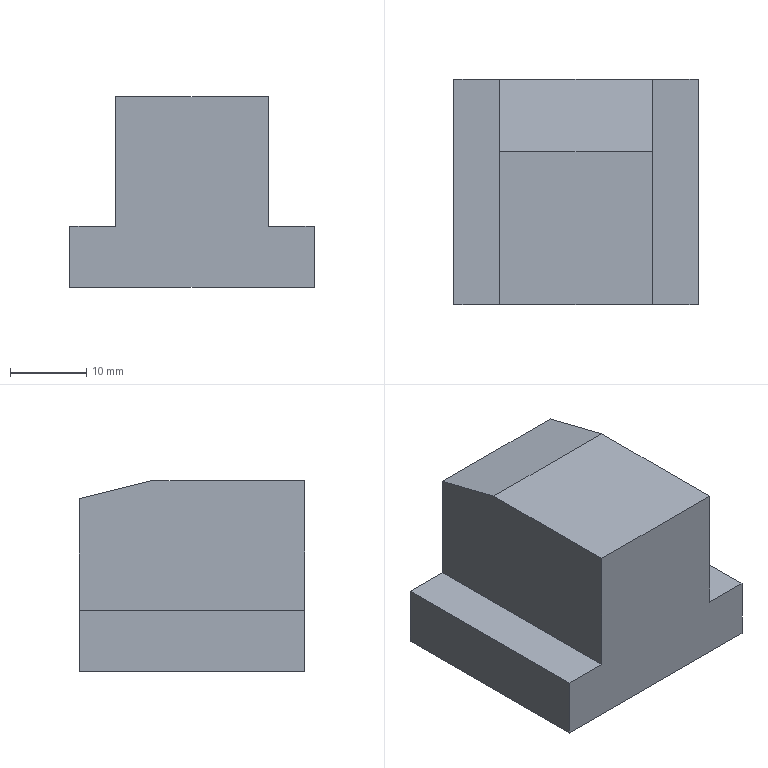Part | STEP file | T-BLOCK2_id178_x_t | 1 solid | 11 faces | box 32 x 29.5 x 25 mm | volume 17357 mm3 | plane 11
STEP:
#1=CARTESIAN_POINT('',(-20.,-40.,235.003));
#2=VERTEX_POINT('',#1);
#3=CARTESIAN_POINT('',(-40.,-40.,235.003));
#4=VERTEX_POINT('',#3);
#5=CARTESIAN_POINT('',(-40.,-40.,235.003));
#6=DIRECTION('',(-1.,0.,0.));
#7=VECTOR('',#6,1.);
#8=LINE('',#5,#7);
#9=EDGE_CURVE('',#2,#4,#8,.T.);
#10=ORIENTED_EDGE('',*,*,#9,.F.);
#11=CARTESIAN_POINT('',(-20.,-30.5,232.634));
#12=VERTEX_POINT('',#11);
#13=CARTESIAN_POINT('',(-20.,-30.5,232.634));
#14=DIRECTION('',(0.,-0.9703,0.2419));
#15=VECTOR('',#14,1.);
#16=LINE('',#13,#15);
#17=EDGE_CURVE('',#12,#2,#16,.T.);
#18=ORIENTED_EDGE('',*,*,#17,.F.);
#19=CARTESIAN_POINT('',(-40.,-30.5,232.634));
#20=VERTEX_POINT('',#19);
#21=CARTESIAN_POINT('',(64.,-30.5,232.634));
#22=DIRECTION('',(1.,0.,0.));
#23=VECTOR('',#22,1.);
#24=LINE('',#21,#23);
#25=EDGE_CURVE('',#20,#12,#24,.T.);
#26=ORIENTED_EDGE('',*,*,#25,.F.);
#27=CARTESIAN_POINT('',(-40.,-40.,235.003));
#28=DIRECTION('',(0.,0.9703,-0.2419));
#29=VECTOR('',#28,1.);
#30=LINE('',#27,#29);
#31=EDGE_CURVE('',#4,#20,#30,.T.);
#32=ORIENTED_EDGE('',*,*,#31,.F.);
#33=EDGE_LOOP('',(#10,#18,#26,#32));
#34=FACE_OUTER_BOUND('',#33,.T.);
#35=CARTESIAN_POINT('',(64.,-40.,235.003));
#36=DIRECTION('',(0.,-0.2419,-0.9703));
#37=DIRECTION('',(0.,0.9703,-0.2419));
#38=AXIS2_PLACEMENT_3D('',#35,#36,#37);
#39=PLANE('',#38);
#40=ADVANCED_FACE('',(#34),#39,.F.);
#41=CARTESIAN_POINT('',(-20.,-60.,235.003));
#42=VERTEX_POINT('',#41);
#43=CARTESIAN_POINT('',(-20.,-60.,235.003));
#44=DIRECTION('',(0.,-1.,0.));
#45=VECTOR('',#44,1.);
#46=LINE('',#43,#45);
#47=EDGE_CURVE('',#2,#42,#46,.T.);
#48=ORIENTED_EDGE('',*,*,#47,.F.);
#49=ORIENTED_EDGE('',*,*,#9,.T.);
#50=CARTESIAN_POINT('',(-40.,-60.,235.003));
#51=VERTEX_POINT('',#50);
#52=CARTESIAN_POINT('',(-40.,-60.,235.003));
#53=DIRECTION('',(0.,1.,0.));
#54=VECTOR('',#53,1.);
#55=LINE('',#52,#54);
#56=EDGE_CURVE('',#51,#4,#55,.T.);
#57=ORIENTED_EDGE('',*,*,#56,.F.);
#58=CARTESIAN_POINT('',(64.,-60.,235.003));
#59=DIRECTION('',(1.,0.,0.));
#60=VECTOR('',#59,1.);
#61=LINE('',#58,#60);
#62=EDGE_CURVE('',#51,#42,#61,.T.);
#63=ORIENTED_EDGE('',*,*,#62,.T.);
#64=EDGE_LOOP('',(#48,#49,#57,#63));
#65=FACE_OUTER_BOUND('',#64,.T.);
#66=CARTESIAN_POINT('',(-40.,-60.,235.003));
#67=DIRECTION('',(0.,0.,1.));
#68=DIRECTION('',(1.,0.,0.));
#69=AXIS2_PLACEMENT_3D('',#66,#67,#68);
#70=PLANE('',#69);
#71=ADVANCED_FACE('',(#65),#70,.T.);
#72=CARTESIAN_POINT('',(-20.,-30.5,218.003));
#73=VERTEX_POINT('',#72);
#74=CARTESIAN_POINT('',(-20.,-30.5,160.003));
#75=DIRECTION('',(0.,0.,-1.));
#76=VECTOR('',#75,1.);
#77=LINE('',#74,#76);
#78=EDGE_CURVE('',#12,#73,#77,.T.);
#79=ORIENTED_EDGE('',*,*,#78,.F.);
#80=ORIENTED_EDGE('',*,*,#17,.T.);
#81=ORIENTED_EDGE('',*,*,#47,.T.);
#82=CARTESIAN_POINT('',(-20.,-60.,218.003));
#83=VERTEX_POINT('',#82);
#84=CARTESIAN_POINT('',(-20.,-60.,160.003));
#85=DIRECTION('',(0.,0.,-1.));
#86=VECTOR('',#85,1.);
#87=LINE('',#84,#86);
#88=EDGE_CURVE('',#42,#83,#87,.T.);
#89=ORIENTED_EDGE('',*,*,#88,.T.);
#90=CARTESIAN_POINT('',(-20.,-60.,218.003));
#91=DIRECTION('',(0.,-1.,0.));
#92=VECTOR('',#91,1.);
#93=LINE('',#90,#92);
#94=EDGE_CURVE('',#73,#83,#93,.T.);
#95=ORIENTED_EDGE('',*,*,#94,.F.);
#96=EDGE_LOOP('',(#79,#80,#81,#89,#95));
#97=FACE_OUTER_BOUND('',#96,.T.);
#98=CARTESIAN_POINT('',(-20.,-60.,235.003));
#99=DIRECTION('',(1.,0.,0.));
#100=DIRECTION('',(0.,0.,-1.));
#101=AXIS2_PLACEMENT_3D('',#98,#99,#100);
#102=PLANE('',#101);
#103=ADVANCED_FACE('',(#97),#102,.T.);
#104=ORIENTED_EDGE('',*,*,#94,.T.);
#105=CARTESIAN_POINT('',(-14.,-60.,218.003));
#106=VERTEX_POINT('',#105);
#107=CARTESIAN_POINT('',(64.,-60.,218.003));
#108=DIRECTION('',(1.,0.,0.));
#109=VECTOR('',#108,1.);
#110=LINE('',#107,#109);
#111=EDGE_CURVE('',#83,#106,#110,.T.);
#112=ORIENTED_EDGE('',*,*,#111,.T.);
#113=CARTESIAN_POINT('',(-14.,-30.5,218.003));
#114=VERTEX_POINT('',#113);
#115=CARTESIAN_POINT('',(-14.,-60.,218.003));
#116=DIRECTION('',(0.,-1.,0.));
#117=VECTOR('',#116,1.);
#118=LINE('',#115,#117);
#119=EDGE_CURVE('',#114,#106,#118,.T.);
#120=ORIENTED_EDGE('',*,*,#119,.F.);
#121=CARTESIAN_POINT('',(64.,-30.5,218.003));
#122=DIRECTION('',(1.,0.,0.));
#123=VECTOR('',#122,1.);
#124=LINE('',#121,#123);
#125=EDGE_CURVE('',#73,#114,#124,.T.);
#126=ORIENTED_EDGE('',*,*,#125,.F.);
#127=EDGE_LOOP('',(#104,#112,#120,#126));
#128=FACE_OUTER_BOUND('',#127,.T.);
#129=CARTESIAN_POINT('',(-20.,-60.,218.003));
#130=DIRECTION('',(0.,0.,1.));
#131=DIRECTION('',(1.,0.,0.));
#132=AXIS2_PLACEMENT_3D('',#129,#130,#131);
#133=PLANE('',#132);
#134=ADVANCED_FACE('',(#128),#133,.T.);
#135=CARTESIAN_POINT('',(-46.,-60.,218.003));
#136=VERTEX_POINT('',#135);
#137=CARTESIAN_POINT('',(-46.,-30.5,218.003));
#138=VERTEX_POINT('',#137);
#139=CARTESIAN_POINT('',(-46.,-60.,218.003));
#140=DIRECTION('',(0.,1.,0.));
#141=VECTOR('',#140,1.);
#142=LINE('',#139,#141);
#143=EDGE_CURVE('',#136,#138,#142,.T.);
#144=ORIENTED_EDGE('',*,*,#143,.F.);
#145=CARTESIAN_POINT('',(-40.,-60.,218.003));
#146=VERTEX_POINT('',#145);
#147=CARTESIAN_POINT('',(64.,-60.,218.003));
#148=DIRECTION('',(1.,0.,0.));
#149=VECTOR('',#148,1.);
#150=LINE('',#147,#149);
#151=EDGE_CURVE('',#136,#146,#150,.T.);
#152=ORIENTED_EDGE('',*,*,#151,.T.);
#153=CARTESIAN_POINT('',(-40.,-30.5,218.003));
#154=VERTEX_POINT('',#153);
#155=CARTESIAN_POINT('',(-40.,-60.,218.003));
#156=DIRECTION('',(0.,-1.,0.));
#157=VECTOR('',#156,1.);
#158=LINE('',#155,#157);
#159=EDGE_CURVE('',#154,#146,#158,.T.);
#160=ORIENTED_EDGE('',*,*,#159,.F.);
#161=CARTESIAN_POINT('',(64.,-30.5,218.003));
#162=DIRECTION('',(1.,0.,0.));
#163=VECTOR('',#162,1.);
#164=LINE('',#161,#163);
#165=EDGE_CURVE('',#138,#154,#164,.T.);
#166=ORIENTED_EDGE('',*,*,#165,.F.);
#167=EDGE_LOOP('',(#144,#152,#160,#166));
#168=FACE_OUTER_BOUND('',#167,.T.);
#169=CARTESIAN_POINT('',(-46.,-60.,218.003));
#170=DIRECTION('',(0.,0.,1.));
#171=DIRECTION('',(1.,0.,0.));
#172=AXIS2_PLACEMENT_3D('',#169,#170,#171);
#173=PLANE('',#172);
#174=ADVANCED_FACE('',(#168),#173,.T.);
#175=ORIENTED_EDGE('',*,*,#56,.T.);
#176=ORIENTED_EDGE('',*,*,#31,.T.);
#177=CARTESIAN_POINT('',(-40.,-30.5,160.003));
#178=DIRECTION('',(0.,0.,1.));
#179=VECTOR('',#178,1.);
#180=LINE('',#177,#179);
#181=EDGE_CURVE('',#154,#20,#180,.T.);
#182=ORIENTED_EDGE('',*,*,#181,.F.);
#183=ORIENTED_EDGE('',*,*,#159,.T.);
#184=CARTESIAN_POINT('',(-40.,-60.,160.003));
#185=DIRECTION('',(0.,0.,1.));
#186=VECTOR('',#185,1.);
#187=LINE('',#184,#186);
#188=EDGE_CURVE('',#146,#51,#187,.T.);
#189=ORIENTED_EDGE('',*,*,#188,.T.);
#190=EDGE_LOOP('',(#175,#176,#182,#183,#189));
#191=FACE_OUTER_BOUND('',#190,.T.);
#192=CARTESIAN_POINT('',(-40.,-60.,218.003));
#193=DIRECTION('',(-1.,0.,0.));
#194=DIRECTION('',(0.,0.,1.));
#195=AXIS2_PLACEMENT_3D('',#192,#193,#194);
#196=PLANE('',#195);
#197=ADVANCED_FACE('',(#191),#196,.T.);
#198=CARTESIAN_POINT('',(-46.,-60.,210.003));
#199=VERTEX_POINT('',#198);
#200=CARTESIAN_POINT('',(-46.,-30.5,210.003));
#201=VERTEX_POINT('',#200);
#202=CARTESIAN_POINT('',(-46.,-60.,210.003));
#203=DIRECTION('',(0.,1.,0.));
#204=VECTOR('',#203,1.);
#205=LINE('',#202,#204);
#206=EDGE_CURVE('',#199,#201,#205,.T.);
#207=ORIENTED_EDGE('',*,*,#206,.F.);
#208=CARTESIAN_POINT('',(-46.,-60.,160.003));
#209=DIRECTION('',(0.,0.,1.));
#210=VECTOR('',#209,1.);
#211=LINE('',#208,#210);
#212=EDGE_CURVE('',#199,#136,#211,.T.);
#213=ORIENTED_EDGE('',*,*,#212,.T.);
#214=ORIENTED_EDGE('',*,*,#143,.T.);
#215=CARTESIAN_POINT('',(-46.,-30.5,160.003));
#216=DIRECTION('',(0.,0.,1.));
#217=VECTOR('',#216,1.);
#218=LINE('',#215,#217);
#219=EDGE_CURVE('',#201,#138,#218,.T.);
#220=ORIENTED_EDGE('',*,*,#219,.F.);
#221=EDGE_LOOP('',(#207,#213,#214,#220));
#222=FACE_OUTER_BOUND('',#221,.T.);
#223=CARTESIAN_POINT('',(-46.,-60.,210.003));
#224=DIRECTION('',(-1.,0.,0.));
#225=DIRECTION('',(0.,0.,1.));
#226=AXIS2_PLACEMENT_3D('',#223,#224,#225);
#227=PLANE('',#226);
#228=ADVANCED_FACE('',(#222),#227,.T.);
#229=ORIENTED_EDGE('',*,*,#181,.T.);
#230=ORIENTED_EDGE('',*,*,#25,.T.);
#231=ORIENTED_EDGE('',*,*,#78,.T.);
#232=ORIENTED_EDGE('',*,*,#125,.T.);
#233=CARTESIAN_POINT('',(-14.,-30.5,210.003));
#234=VERTEX_POINT('',#233);
#235=CARTESIAN_POINT('',(-14.,-30.5,218.003));
#236=DIRECTION('',(0.,0.,1.));
#237=VECTOR('',#236,1.);
#238=LINE('',#235,#237);
#239=EDGE_CURVE('',#234,#114,#238,.T.);
#240=ORIENTED_EDGE('',*,*,#239,.F.);
#241=CARTESIAN_POINT('',(-14.,-30.5,210.003));
#242=DIRECTION('',(1.,0.,0.));
#243=VECTOR('',#242,1.);
#244=LINE('',#241,#243);
#245=EDGE_CURVE('',#201,#234,#244,.T.);
#246=ORIENTED_EDGE('',*,*,#245,.F.);
#247=ORIENTED_EDGE('',*,*,#219,.T.);
#248=ORIENTED_EDGE('',*,*,#165,.T.);
#249=EDGE_LOOP('',(#229,#230,#231,#232,#240,#246,#247,#248));
#250=FACE_OUTER_BOUND('',#249,.T.);
#251=CARTESIAN_POINT('',(64.,-30.5,160.003));
#252=DIRECTION('',(0.,1.,0.));
#253=DIRECTION('',(0.,0.,1.));
#254=AXIS2_PLACEMENT_3D('',#251,#252,#253);
#255=PLANE('',#254);
#256=ADVANCED_FACE('',(#250),#255,.T.);
#257=ORIENTED_EDGE('',*,*,#119,.T.);
#258=CARTESIAN_POINT('',(-14.,-60.,210.003));
#259=VERTEX_POINT('',#258);
#260=CARTESIAN_POINT('',(-14.,-60.,160.003));
#261=DIRECTION('',(0.,0.,-1.));
#262=VECTOR('',#261,1.);
#263=LINE('',#260,#262);
#264=EDGE_CURVE('',#106,#259,#263,.T.);
#265=ORIENTED_EDGE('',*,*,#264,.T.);
#266=CARTESIAN_POINT('',(-14.,-60.,210.003));
#267=DIRECTION('',(0.,-1.,0.));
#268=VECTOR('',#267,1.);
#269=LINE('',#266,#268);
#270=EDGE_CURVE('',#234,#259,#269,.T.);
#271=ORIENTED_EDGE('',*,*,#270,.F.);
#272=ORIENTED_EDGE('',*,*,#239,.T.);
#273=EDGE_LOOP('',(#257,#265,#271,#272));
#274=FACE_OUTER_BOUND('',#273,.T.);
#275=CARTESIAN_POINT('',(-14.,-60.,218.003));
#276=DIRECTION('',(1.,0.,0.));
#277=DIRECTION('',(0.,0.,-1.));
#278=AXIS2_PLACEMENT_3D('',#275,#276,#277);
#279=PLANE('',#278);
#280=ADVANCED_FACE('',(#274),#279,.T.);
#281=ORIENTED_EDGE('',*,*,#151,.F.);
#282=ORIENTED_EDGE('',*,*,#212,.F.);
#283=CARTESIAN_POINT('',(-14.,-60.,210.003));
#284=DIRECTION('',(-1.,0.,0.));
#285=VECTOR('',#284,1.);
#286=LINE('',#283,#285);
#287=EDGE_CURVE('',#259,#199,#286,.T.);
#288=ORIENTED_EDGE('',*,*,#287,.F.);
#289=ORIENTED_EDGE('',*,*,#264,.F.);
#290=ORIENTED_EDGE('',*,*,#111,.F.);
#291=ORIENTED_EDGE('',*,*,#88,.F.);
#292=ORIENTED_EDGE('',*,*,#62,.F.);
#293=ORIENTED_EDGE('',*,*,#188,.F.);
#294=EDGE_LOOP('',(#281,#282,#288,#289,#290,#291,#292,#293));
#295=FACE_OUTER_BOUND('',#294,.T.);
#296=CARTESIAN_POINT('',(64.,-60.,160.003));
#297=DIRECTION('',(0.,1.,0.));
#298=DIRECTION('',(0.,0.,1.));
#299=AXIS2_PLACEMENT_3D('',#296,#297,#298);
#300=PLANE('',#299);
#301=ADVANCED_FACE('',(#295),#300,.F.);
#302=ORIENTED_EDGE('',*,*,#270,.T.);
#303=ORIENTED_EDGE('',*,*,#287,.T.);
#304=ORIENTED_EDGE('',*,*,#206,.T.);
#305=ORIENTED_EDGE('',*,*,#245,.T.);
#306=EDGE_LOOP('',(#302,#303,#304,#305));
#307=FACE_OUTER_BOUND('',#306,.T.);
#308=CARTESIAN_POINT('',(-14.,-60.,210.003));
#309=DIRECTION('',(0.,0.,-1.));
#310=DIRECTION('',(-1.,0.,0.));
#311=AXIS2_PLACEMENT_3D('',#308,#309,#310);
#312=PLANE('',#311);
#313=ADVANCED_FACE('',(#307),#312,.T.);
#314=CLOSED_SHELL('',(#40,#71,#103,#134,#174,#197,#228,#256,#280,#301,#313));
#315=MANIFOLD_SOLID_BREP('',#314);
#316=(LENGTH_UNIT()NAMED_UNIT(*)SI_UNIT(.MILLI.,.METRE.));
#317=UNCERTAINTY_MEASURE_WITH_UNIT(LENGTH_MEASURE(0.00002),#316,'','');
#318=(NAMED_UNIT(*)PLANE_ANGLE_UNIT()SI_UNIT($,.RADIAN.));
#319=PLANE_ANGLE_MEASURE_WITH_UNIT(PLANE_ANGLE_MEASURE(0.01745),#318);
#320=DIMENSIONAL_EXPONENTS(0.,0.,0.,0.,0.,0.,0.);
#321=(CONVERSION_BASED_UNIT('DEGREE',#319)NAMED_UNIT(#320)PLANE_ANGLE_UNIT());
#322=(NAMED_UNIT(*)SI_UNIT($,.STERADIAN.)SOLID_ANGLE_UNIT());
#323=(GEOMETRIC_REPRESENTATION_CONTEXT(3)GLOBAL_UNCERTAINTY_ASSIGNED_CONTEXT((#317))GLOBAL_UNIT_ASSIGNED_CONTEXT((#316,#321,#322))REPRESENTATION_CONTEXT('',''));
#324=ADVANCED_BREP_SHAPE_REPRESENTATION('',(#315),#323);